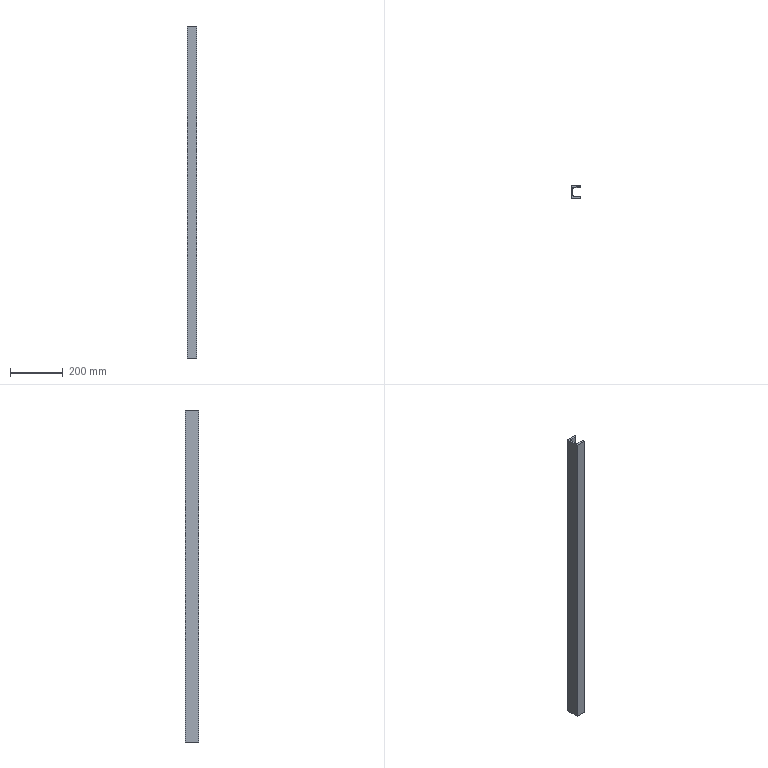Part | STEP file | DIN 1026-1 U 50 1785357045389 | 1 solid | 14 faces | box 38 x 50 x 1265 mm | volume 900372 mm3 | plane 10 | cylinder 4 | commonest cylinder face diameters 7 x2 14 x2
STEP:
#1=CARTESIAN_POINT('',(5.,-10.418,1314.813));
#2=VERTEX_POINT('',#1);
#3=CARTESIAN_POINT('',(11.442,-17.395,1314.813));
#4=VERTEX_POINT('',#3);
#5=CARTESIAN_POINT('',(12.,-10.418,1314.813));
#6=DIRECTION('',(0.,0.,1.));
#7=DIRECTION('',(-1.,0.,0.));
#8=AXIS2_PLACEMENT_3D('',#5,#6,#7);
#9=CIRCLE('',#8,7.);
#10=EDGE_CURVE('',#2,#4,#9,.T.);
#11=ORIENTED_EDGE('',*,*,#10,.T.);
#12=CARTESIAN_POINT('',(11.442,-17.395,50.));
#13=VERTEX_POINT('',#12);
#14=CARTESIAN_POINT('',(11.442,-17.395,0.));
#15=DIRECTION('',(0.,0.,1.));
#16=VECTOR('',#15,10.);
#17=LINE('',#14,#16);
#18=EDGE_CURVE('',#13,#4,#17,.T.);
#19=ORIENTED_EDGE('',*,*,#18,.F.);
#20=CARTESIAN_POINT('',(5.,-10.418,50.));
#21=VERTEX_POINT('',#20);
#22=CARTESIAN_POINT('',(12.,-10.418,50.));
#23=DIRECTION('',(0.,0.,1.));
#24=DIRECTION('',(-1.,0.,0.));
#25=AXIS2_PLACEMENT_3D('',#22,#23,#24);
#26=CIRCLE('',#25,7.);
#27=EDGE_CURVE('',#21,#13,#26,.T.);
#28=ORIENTED_EDGE('',*,*,#27,.F.);
#29=CARTESIAN_POINT('',(5.,-10.418,0.));
#30=DIRECTION('',(0.,0.,1.));
#31=VECTOR('',#30,10.);
#32=LINE('',#29,#31);
#33=EDGE_CURVE('',#21,#2,#32,.T.);
#34=ORIENTED_EDGE('',*,*,#33,.T.);
#35=EDGE_LOOP('',(#11,#19,#28,#34));
#36=FACE_OUTER_BOUND('',#35,.T.);
#37=CARTESIAN_POINT('',(12.,-10.418,0.));
#38=DIRECTION('',(0.,0.,1.));
#39=DIRECTION('',(-1.,0.,0.));
#40=AXIS2_PLACEMENT_3D('',#37,#38,#39);
#41=CYLINDRICAL_SURFACE('',#40,7.);
#42=ADVANCED_FACE('',(#36),#41,.F.);
#43=CARTESIAN_POINT('',(34.779,-19.262,1314.813));
#44=VERTEX_POINT('',#43);
#45=CARTESIAN_POINT('',(14.505,-17.64,1314.813));
#46=DIRECTION('',(0.9968,-0.07975,0.));
#47=VECTOR('',#46,10.);
#48=LINE('',#45,#47);
#49=EDGE_CURVE('',#4,#44,#48,.T.);
#50=ORIENTED_EDGE('',*,*,#49,.T.);
#51=CARTESIAN_POINT('',(34.779,-19.262,50.));
#52=VERTEX_POINT('',#51);
#53=CARTESIAN_POINT('',(34.779,-19.262,0.));
#54=DIRECTION('',(0.,0.,1.));
#55=VECTOR('',#54,10.);
#56=LINE('',#53,#55);
#57=EDGE_CURVE('',#52,#44,#56,.T.);
#58=ORIENTED_EDGE('',*,*,#57,.F.);
#59=CARTESIAN_POINT('',(14.505,-17.64,50.));
#60=DIRECTION('',(0.9968,-0.07975,0.));
#61=VECTOR('',#60,10.);
#62=LINE('',#59,#61);
#63=EDGE_CURVE('',#13,#52,#62,.T.);
#64=ORIENTED_EDGE('',*,*,#63,.F.);
#65=ORIENTED_EDGE('',*,*,#18,.T.);
#66=EDGE_LOOP('',(#50,#58,#64,#65));
#67=FACE_OUTER_BOUND('',#66,.T.);
#68=CARTESIAN_POINT('',(11.442,-17.395,0.));
#69=DIRECTION('',(0.07975,0.9968,0.));
#70=DIRECTION('',(0.,0.,1.));
#71=AXIS2_PLACEMENT_3D('',#68,#69,#70);
#72=PLANE('',#71);
#73=ADVANCED_FACE('',(#67),#72,.T.);
#74=CARTESIAN_POINT('',(38.,-22.751,1314.813));
#75=VERTEX_POINT('',#74);
#76=CARTESIAN_POINT('',(34.5,-22.751,1314.813));
#77=DIRECTION('',(0.,0.,-1.));
#78=DIRECTION('',(-1.,0.,0.));
#79=AXIS2_PLACEMENT_3D('',#76,#77,#78);
#80=CIRCLE('',#79,3.5);
#81=EDGE_CURVE('',#44,#75,#80,.T.);
#82=ORIENTED_EDGE('',*,*,#81,.T.);
#83=CARTESIAN_POINT('',(38.,-22.751,50.));
#84=VERTEX_POINT('',#83);
#85=CARTESIAN_POINT('',(38.,-22.751,0.));
#86=DIRECTION('',(0.,0.,1.));
#87=VECTOR('',#86,10.);
#88=LINE('',#85,#87);
#89=EDGE_CURVE('',#84,#75,#88,.T.);
#90=ORIENTED_EDGE('',*,*,#89,.F.);
#91=CARTESIAN_POINT('',(34.5,-22.751,50.));
#92=DIRECTION('',(0.,0.,-1.));
#93=DIRECTION('',(-1.,0.,0.));
#94=AXIS2_PLACEMENT_3D('',#91,#92,#93);
#95=CIRCLE('',#94,3.5);
#96=EDGE_CURVE('',#52,#84,#95,.T.);
#97=ORIENTED_EDGE('',*,*,#96,.F.);
#98=ORIENTED_EDGE('',*,*,#57,.T.);
#99=EDGE_LOOP('',(#82,#90,#97,#98));
#100=FACE_OUTER_BOUND('',#99,.T.);
#101=CARTESIAN_POINT('',(34.5,-22.751,0.));
#102=DIRECTION('',(0.,0.,1.));
#103=DIRECTION('',(-1.,0.,0.));
#104=AXIS2_PLACEMENT_3D('',#101,#102,#103);
#105=CYLINDRICAL_SURFACE('',#104,3.5);
#106=ADVANCED_FACE('',(#100),#105,.T.);
#107=CARTESIAN_POINT('',(38.,-25.,1314.813));
#108=VERTEX_POINT('',#107);
#109=CARTESIAN_POINT('',(38.,-11.376,1314.813));
#110=DIRECTION('',(0.,-1.,0.));
#111=VECTOR('',#110,10.);
#112=LINE('',#109,#111);
#113=EDGE_CURVE('',#75,#108,#112,.T.);
#114=ORIENTED_EDGE('',*,*,#113,.T.);
#115=CARTESIAN_POINT('',(38.,-25.,50.));
#116=VERTEX_POINT('',#115);
#117=CARTESIAN_POINT('',(38.,-25.,0.));
#118=DIRECTION('',(0.,0.,1.));
#119=VECTOR('',#118,10.);
#120=LINE('',#117,#119);
#121=EDGE_CURVE('',#116,#108,#120,.T.);
#122=ORIENTED_EDGE('',*,*,#121,.F.);
#123=CARTESIAN_POINT('',(38.,-11.376,50.));
#124=DIRECTION('',(0.,-1.,0.));
#125=VECTOR('',#124,10.);
#126=LINE('',#123,#125);
#127=EDGE_CURVE('',#84,#116,#126,.T.);
#128=ORIENTED_EDGE('',*,*,#127,.F.);
#129=ORIENTED_EDGE('',*,*,#89,.T.);
#130=EDGE_LOOP('',(#114,#122,#128,#129));
#131=FACE_OUTER_BOUND('',#130,.T.);
#132=CARTESIAN_POINT('',(38.,-22.751,0.));
#133=DIRECTION('',(1.,0.,0.));
#134=DIRECTION('',(0.,0.,-1.));
#135=AXIS2_PLACEMENT_3D('',#132,#133,#134);
#136=PLANE('',#135);
#137=ADVANCED_FACE('',(#131),#136,.T.);
#138=CARTESIAN_POINT('',(0.,-25.,1314.813));
#139=VERTEX_POINT('',#138);
#140=CARTESIAN_POINT('',(28.5,-25.,1314.813));
#141=DIRECTION('',(-1.,0.,0.));
#142=VECTOR('',#141,10.);
#143=LINE('',#140,#142);
#144=EDGE_CURVE('',#108,#139,#143,.T.);
#145=ORIENTED_EDGE('',*,*,#144,.T.);
#146=CARTESIAN_POINT('',(0.,-25.,50.));
#147=VERTEX_POINT('',#146);
#148=CARTESIAN_POINT('',(0.,-25.,0.));
#149=DIRECTION('',(0.,0.,1.));
#150=VECTOR('',#149,10.);
#151=LINE('',#148,#150);
#152=EDGE_CURVE('',#147,#139,#151,.T.);
#153=ORIENTED_EDGE('',*,*,#152,.F.);
#154=CARTESIAN_POINT('',(28.5,-25.,50.));
#155=DIRECTION('',(-1.,0.,0.));
#156=VECTOR('',#155,10.);
#157=LINE('',#154,#156);
#158=EDGE_CURVE('',#116,#147,#157,.T.);
#159=ORIENTED_EDGE('',*,*,#158,.F.);
#160=ORIENTED_EDGE('',*,*,#121,.T.);
#161=EDGE_LOOP('',(#145,#153,#159,#160));
#162=FACE_OUTER_BOUND('',#161,.T.);
#163=CARTESIAN_POINT('',(38.,-25.,0.));
#164=DIRECTION('',(0.,-1.,0.));
#165=DIRECTION('',(0.,0.,-1.));
#166=AXIS2_PLACEMENT_3D('',#163,#164,#165);
#167=PLANE('',#166);
#168=ADVANCED_FACE('',(#162),#167,.T.);
#169=CARTESIAN_POINT('',(0.,25.,1314.813));
#170=VERTEX_POINT('',#169);
#171=CARTESIAN_POINT('',(0.,0.,1314.813));
#172=DIRECTION('',(0.,1.,0.));
#173=VECTOR('',#172,10.);
#174=LINE('',#171,#173);
#175=EDGE_CURVE('',#139,#170,#174,.T.);
#176=ORIENTED_EDGE('',*,*,#175,.T.);
#177=CARTESIAN_POINT('',(0.,25.,50.));
#178=VERTEX_POINT('',#177);
#179=CARTESIAN_POINT('',(0.,25.,0.));
#180=DIRECTION('',(0.,0.,1.));
#181=VECTOR('',#180,10.);
#182=LINE('',#179,#181);
#183=EDGE_CURVE('',#178,#170,#182,.T.);
#184=ORIENTED_EDGE('',*,*,#183,.F.);
#185=CARTESIAN_POINT('',(0.,0.,50.));
#186=DIRECTION('',(0.,1.,0.));
#187=VECTOR('',#186,10.);
#188=LINE('',#185,#187);
#189=EDGE_CURVE('',#147,#178,#188,.T.);
#190=ORIENTED_EDGE('',*,*,#189,.F.);
#191=ORIENTED_EDGE('',*,*,#152,.T.);
#192=EDGE_LOOP('',(#176,#184,#190,#191));
#193=FACE_OUTER_BOUND('',#192,.T.);
#194=CARTESIAN_POINT('',(0.,0.,0.));
#195=DIRECTION('',(-1.,0.,0.));
#196=DIRECTION('',(0.,0.,1.));
#197=AXIS2_PLACEMENT_3D('',#194,#195,#196);
#198=PLANE('',#197);
#199=ADVANCED_FACE('',(#193),#198,.T.);
#200=CARTESIAN_POINT('',(38.,25.,1314.813));
#201=VERTEX_POINT('',#200);
#202=CARTESIAN_POINT('',(9.5,25.,1314.813));
#203=DIRECTION('',(1.,0.,0.));
#204=VECTOR('',#203,10.);
#205=LINE('',#202,#204);
#206=EDGE_CURVE('',#170,#201,#205,.T.);
#207=ORIENTED_EDGE('',*,*,#206,.T.);
#208=CARTESIAN_POINT('',(38.,25.,50.));
#209=VERTEX_POINT('',#208);
#210=CARTESIAN_POINT('',(38.,25.,0.));
#211=DIRECTION('',(0.,0.,1.));
#212=VECTOR('',#211,10.);
#213=LINE('',#210,#212);
#214=EDGE_CURVE('',#209,#201,#213,.T.);
#215=ORIENTED_EDGE('',*,*,#214,.F.);
#216=CARTESIAN_POINT('',(9.5,25.,50.));
#217=DIRECTION('',(1.,0.,0.));
#218=VECTOR('',#217,10.);
#219=LINE('',#216,#218);
#220=EDGE_CURVE('',#178,#209,#219,.T.);
#221=ORIENTED_EDGE('',*,*,#220,.F.);
#222=ORIENTED_EDGE('',*,*,#183,.T.);
#223=EDGE_LOOP('',(#207,#215,#221,#222));
#224=FACE_OUTER_BOUND('',#223,.T.);
#225=CARTESIAN_POINT('',(0.,25.,0.));
#226=DIRECTION('',(0.,1.,0.));
#227=DIRECTION('',(0.,0.,1.));
#228=AXIS2_PLACEMENT_3D('',#225,#226,#227);
#229=PLANE('',#228);
#230=ADVANCED_FACE('',(#224),#229,.T.);
#231=CARTESIAN_POINT('',(38.,22.751,1314.813));
#232=VERTEX_POINT('',#231);
#233=CARTESIAN_POINT('',(38.,12.5,1314.813));
#234=DIRECTION('',(0.,-1.,0.));
#235=VECTOR('',#234,10.);
#236=LINE('',#233,#235);
#237=EDGE_CURVE('',#201,#232,#236,.T.);
#238=ORIENTED_EDGE('',*,*,#237,.T.);
#239=CARTESIAN_POINT('',(38.,22.751,50.));
#240=VERTEX_POINT('',#239);
#241=CARTESIAN_POINT('',(38.,22.751,0.));
#242=DIRECTION('',(0.,0.,1.));
#243=VECTOR('',#242,10.);
#244=LINE('',#241,#243);
#245=EDGE_CURVE('',#240,#232,#244,.T.);
#246=ORIENTED_EDGE('',*,*,#245,.F.);
#247=CARTESIAN_POINT('',(38.,12.5,50.));
#248=DIRECTION('',(0.,-1.,0.));
#249=VECTOR('',#248,10.);
#250=LINE('',#247,#249);
#251=EDGE_CURVE('',#209,#240,#250,.T.);
#252=ORIENTED_EDGE('',*,*,#251,.F.);
#253=ORIENTED_EDGE('',*,*,#214,.T.);
#254=EDGE_LOOP('',(#238,#246,#252,#253));
#255=FACE_OUTER_BOUND('',#254,.T.);
#256=CARTESIAN_POINT('',(38.,25.,0.));
#257=DIRECTION('',(1.,0.,0.));
#258=DIRECTION('',(0.,0.,-1.));
#259=AXIS2_PLACEMENT_3D('',#256,#257,#258);
#260=PLANE('',#259);
#261=ADVANCED_FACE('',(#255),#260,.T.);
#262=CARTESIAN_POINT('',(34.779,19.262,1314.813));
#263=VERTEX_POINT('',#262);
#264=CARTESIAN_POINT('',(34.5,22.751,1314.813));
#265=DIRECTION('',(0.,0.,-1.));
#266=DIRECTION('',(-0.07975,0.9968,0.));
#267=AXIS2_PLACEMENT_3D('',#264,#265,#266);
#268=CIRCLE('',#267,3.5);
#269=EDGE_CURVE('',#232,#263,#268,.T.);
#270=ORIENTED_EDGE('',*,*,#269,.T.);
#271=CARTESIAN_POINT('',(34.779,19.262,50.));
#272=VERTEX_POINT('',#271);
#273=CARTESIAN_POINT('',(34.779,19.262,0.));
#274=DIRECTION('',(0.,0.,1.));
#275=VECTOR('',#274,10.);
#276=LINE('',#273,#275);
#277=EDGE_CURVE('',#272,#263,#276,.T.);
#278=ORIENTED_EDGE('',*,*,#277,.F.);
#279=CARTESIAN_POINT('',(34.5,22.751,50.));
#280=DIRECTION('',(0.,0.,-1.));
#281=DIRECTION('',(-0.07975,0.9968,0.));
#282=AXIS2_PLACEMENT_3D('',#279,#280,#281);
#283=CIRCLE('',#282,3.5);
#284=EDGE_CURVE('',#240,#272,#283,.T.);
#285=ORIENTED_EDGE('',*,*,#284,.F.);
#286=ORIENTED_EDGE('',*,*,#245,.T.);
#287=EDGE_LOOP('',(#270,#278,#285,#286));
#288=FACE_OUTER_BOUND('',#287,.T.);
#289=CARTESIAN_POINT('',(34.5,22.751,0.));
#290=DIRECTION('',(0.,0.,1.));
#291=DIRECTION('',(-0.07975,0.9968,0.));
#292=AXIS2_PLACEMENT_3D('',#289,#290,#291);
#293=CYLINDRICAL_SURFACE('',#292,3.5);
#294=ADVANCED_FACE('',(#288),#293,.T.);
#295=CARTESIAN_POINT('',(11.442,17.395,1314.813));
#296=VERTEX_POINT('',#295);
#297=CARTESIAN_POINT('',(26.174,18.574,1314.813));
#298=DIRECTION('',(-0.9968,-0.07975,0.));
#299=VECTOR('',#298,10.);
#300=LINE('',#297,#299);
#301=EDGE_CURVE('',#263,#296,#300,.T.);
#302=ORIENTED_EDGE('',*,*,#301,.T.);
#303=CARTESIAN_POINT('',(11.442,17.395,50.));
#304=VERTEX_POINT('',#303);
#305=CARTESIAN_POINT('',(11.442,17.395,0.));
#306=DIRECTION('',(0.,0.,1.));
#307=VECTOR('',#306,10.);
#308=LINE('',#305,#307);
#309=EDGE_CURVE('',#304,#296,#308,.T.);
#310=ORIENTED_EDGE('',*,*,#309,.F.);
#311=CARTESIAN_POINT('',(26.174,18.574,50.));
#312=DIRECTION('',(-0.9968,-0.07975,0.));
#313=VECTOR('',#312,10.);
#314=LINE('',#311,#313);
#315=EDGE_CURVE('',#272,#304,#314,.T.);
#316=ORIENTED_EDGE('',*,*,#315,.F.);
#317=ORIENTED_EDGE('',*,*,#277,.T.);
#318=EDGE_LOOP('',(#302,#310,#316,#317));
#319=FACE_OUTER_BOUND('',#318,.T.);
#320=CARTESIAN_POINT('',(34.779,19.262,0.));
#321=DIRECTION('',(0.07975,-0.9968,0.));
#322=DIRECTION('',(0.,0.,-1.));
#323=AXIS2_PLACEMENT_3D('',#320,#321,#322);
#324=PLANE('',#323);
#325=ADVANCED_FACE('',(#319),#324,.T.);
#326=CARTESIAN_POINT('',(5.,10.418,1314.813));
#327=VERTEX_POINT('',#326);
#328=CARTESIAN_POINT('',(12.,10.418,1314.813));
#329=DIRECTION('',(0.,0.,1.));
#330=DIRECTION('',(-0.07975,0.9968,0.));
#331=AXIS2_PLACEMENT_3D('',#328,#329,#330);
#332=CIRCLE('',#331,7.);
#333=EDGE_CURVE('',#296,#327,#332,.T.);
#334=ORIENTED_EDGE('',*,*,#333,.T.);
#335=CARTESIAN_POINT('',(5.,10.418,50.));
#336=VERTEX_POINT('',#335);
#337=CARTESIAN_POINT('',(5.,10.418,0.));
#338=DIRECTION('',(0.,0.,1.));
#339=VECTOR('',#338,10.);
#340=LINE('',#337,#339);
#341=EDGE_CURVE('',#336,#327,#340,.T.);
#342=ORIENTED_EDGE('',*,*,#341,.F.);
#343=CARTESIAN_POINT('',(12.,10.418,50.));
#344=DIRECTION('',(0.,0.,1.));
#345=DIRECTION('',(-0.07975,0.9968,0.));
#346=AXIS2_PLACEMENT_3D('',#343,#344,#345);
#347=CIRCLE('',#346,7.);
#348=EDGE_CURVE('',#304,#336,#347,.T.);
#349=ORIENTED_EDGE('',*,*,#348,.F.);
#350=ORIENTED_EDGE('',*,*,#309,.T.);
#351=EDGE_LOOP('',(#334,#342,#349,#350));
#352=FACE_OUTER_BOUND('',#351,.T.);
#353=CARTESIAN_POINT('',(12.,10.418,0.));
#354=DIRECTION('',(0.,0.,1.));
#355=DIRECTION('',(-0.07975,0.9968,0.));
#356=AXIS2_PLACEMENT_3D('',#353,#354,#355);
#357=CYLINDRICAL_SURFACE('',#356,7.);
#358=ADVANCED_FACE('',(#352),#357,.F.);
#359=CARTESIAN_POINT('',(5.,0.,1314.813));
#360=DIRECTION('',(0.,-1.,0.));
#361=VECTOR('',#360,10.);
#362=LINE('',#359,#361);
#363=EDGE_CURVE('',#327,#2,#362,.T.);
#364=ORIENTED_EDGE('',*,*,#363,.T.);
#365=ORIENTED_EDGE('',*,*,#33,.F.);
#366=CARTESIAN_POINT('',(5.,0.,50.));
#367=DIRECTION('',(0.,-1.,0.));
#368=VECTOR('',#367,10.);
#369=LINE('',#366,#368);
#370=EDGE_CURVE('',#336,#21,#369,.T.);
#371=ORIENTED_EDGE('',*,*,#370,.F.);
#372=ORIENTED_EDGE('',*,*,#341,.T.);
#373=EDGE_LOOP('',(#364,#365,#371,#372));
#374=FACE_OUTER_BOUND('',#373,.T.);
#375=CARTESIAN_POINT('',(5.,0.,0.));
#376=DIRECTION('',(1.,0.,0.));
#377=DIRECTION('',(0.,0.,-1.));
#378=AXIS2_PLACEMENT_3D('',#375,#376,#377);
#379=PLANE('',#378);
#380=ADVANCED_FACE('',(#374),#379,.T.);
#381=ORIENTED_EDGE('',*,*,#220,.T.);
#382=ORIENTED_EDGE('',*,*,#251,.T.);
#383=ORIENTED_EDGE('',*,*,#284,.T.);
#384=ORIENTED_EDGE('',*,*,#315,.T.);
#385=ORIENTED_EDGE('',*,*,#348,.T.);
#386=ORIENTED_EDGE('',*,*,#370,.T.);
#387=ORIENTED_EDGE('',*,*,#27,.T.);
#388=ORIENTED_EDGE('',*,*,#63,.T.);
#389=ORIENTED_EDGE('',*,*,#96,.T.);
#390=ORIENTED_EDGE('',*,*,#127,.T.);
#391=ORIENTED_EDGE('',*,*,#158,.T.);
#392=ORIENTED_EDGE('',*,*,#189,.T.);
#393=EDGE_LOOP('',(#381,#382,#383,#384,#385,#386,#387,#388,#389,#390,#391,#392));
#394=FACE_OUTER_BOUND('',#393,.T.);
#395=CARTESIAN_POINT('',(19.,0.,50.));
#396=DIRECTION('',(0.,0.,1.));
#397=DIRECTION('',(1.,0.,0.));
#398=AXIS2_PLACEMENT_3D('',#395,#396,#397);
#399=PLANE('',#398);
#400=ADVANCED_FACE('',(#394),#399,.F.);
#401=ORIENTED_EDGE('',*,*,#206,.F.);
#402=ORIENTED_EDGE('',*,*,#175,.F.);
#403=ORIENTED_EDGE('',*,*,#144,.F.);
#404=ORIENTED_EDGE('',*,*,#113,.F.);
#405=ORIENTED_EDGE('',*,*,#81,.F.);
#406=ORIENTED_EDGE('',*,*,#49,.F.);
#407=ORIENTED_EDGE('',*,*,#10,.F.);
#408=ORIENTED_EDGE('',*,*,#363,.F.);
#409=ORIENTED_EDGE('',*,*,#333,.F.);
#410=ORIENTED_EDGE('',*,*,#301,.F.);
#411=ORIENTED_EDGE('',*,*,#269,.F.);
#412=ORIENTED_EDGE('',*,*,#237,.F.);
#413=EDGE_LOOP('',(#401,#402,#403,#404,#405,#406,#407,#408,#409,#410,#411,#412));
#414=FACE_OUTER_BOUND('',#413,.T.);
#415=CARTESIAN_POINT('',(19.,0.,1314.813));
#416=DIRECTION('',(0.,0.,1.));
#417=DIRECTION('',(1.,0.,0.));
#418=AXIS2_PLACEMENT_3D('',#415,#416,#417);
#419=PLANE('',#418);
#420=ADVANCED_FACE('',(#414),#419,.T.);
#421=CLOSED_SHELL('',(#42,#73,#106,#137,#168,#199,#230,#261,#294,#325,#358,#380,#400,#420));
#422=MANIFOLD_SOLID_BREP('',#421);
#423=(LENGTH_UNIT()NAMED_UNIT(*)SI_UNIT(.MILLI.,.METRE.));
#424=UNCERTAINTY_MEASURE_WITH_UNIT(LENGTH_MEASURE(0.01),#423,'','');
#425=(NAMED_UNIT(*)PLANE_ANGLE_UNIT()SI_UNIT($,.RADIAN.));
#426=(NAMED_UNIT(*)SI_UNIT($,.STERADIAN.)SOLID_ANGLE_UNIT());
#427=(GEOMETRIC_REPRESENTATION_CONTEXT(3)GLOBAL_UNCERTAINTY_ASSIGNED_CONTEXT((#424))GLOBAL_UNIT_ASSIGNED_CONTEXT((#423,#425,#426))REPRESENTATION_CONTEXT('',''));
#428=ADVANCED_BREP_SHAPE_REPRESENTATION('',(#422),#427);